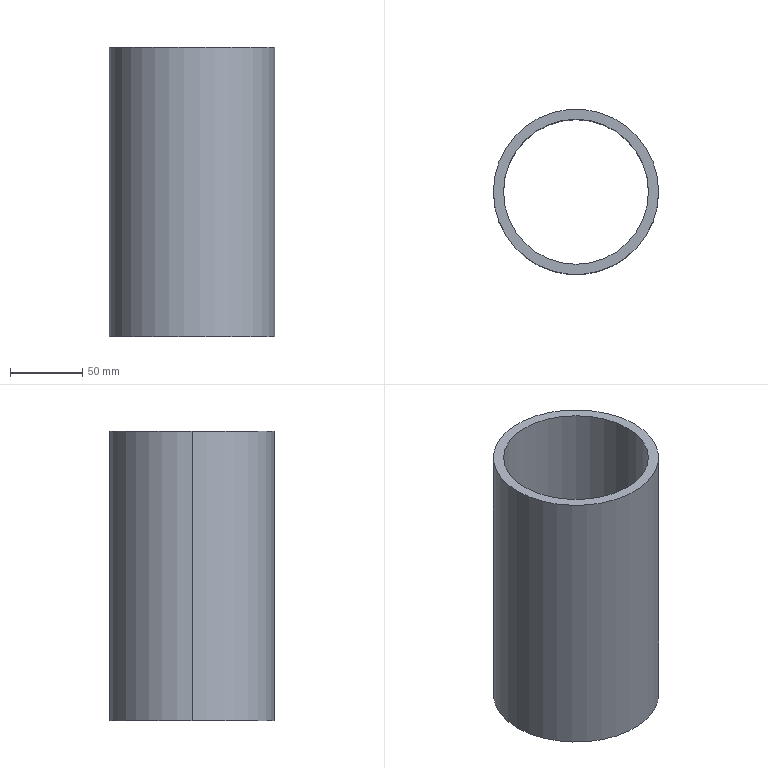Part | SolidWorks | features Extrusion 1, RefAxis 1 | 1 solid | 6 faces | box 114 x 114 x 200 mm | volume 470611 mm3 | cylinder 4 | plane 2 | commonest cylinder face diameters 100 x2 114 x2
STEP:
#1=CARTESIAN_POINT('',(-50.,0.,200.));
#2=VERTEX_POINT('',#1);
#3=CARTESIAN_POINT('',(50.,0.,200.));
#4=VERTEX_POINT('',#3);
#5=CARTESIAN_POINT('',(0.,0.,200.));
#6=DIRECTION('',(0.,0.,1.));
#7=DIRECTION('',(1.,0.,0.));
#8=AXIS2_PLACEMENT_3D('',#5,#6,#7);
#9=CIRCLE('',#8,50.);
#10=EDGE_CURVE('',#2,#4,#9,.T.);
#11=ORIENTED_EDGE('',*,*,#10,.T.);
#12=CARTESIAN_POINT('',(50.,0.,0.));
#13=VERTEX_POINT('',#12);
#14=CARTESIAN_POINT('',(50.,0.,200.));
#15=DIRECTION('',(0.,0.,-1.));
#16=VECTOR('',#15,1000.);
#17=LINE('',#14,#16);
#18=EDGE_CURVE('',#4,#13,#17,.T.);
#19=ORIENTED_EDGE('',*,*,#18,.T.);
#20=CARTESIAN_POINT('',(-50.,0.,0.));
#21=VERTEX_POINT('',#20);
#22=CARTESIAN_POINT('',(0.,0.,0.));
#23=DIRECTION('',(0.,0.,1.));
#24=DIRECTION('',(1.,0.,0.));
#25=AXIS2_PLACEMENT_3D('',#22,#23,#24);
#26=CIRCLE('',#25,50.);
#27=EDGE_CURVE('',#21,#13,#26,.T.);
#28=ORIENTED_EDGE('',*,*,#27,.F.);
#29=CARTESIAN_POINT('',(-50.,0.,200.));
#30=DIRECTION('',(0.,0.,-1.));
#31=VECTOR('',#30,1000.);
#32=LINE('',#29,#31);
#33=EDGE_CURVE('',#2,#21,#32,.T.);
#34=ORIENTED_EDGE('',*,*,#33,.F.);
#35=EDGE_LOOP('',(#11,#19,#28,#34));
#36=FACE_OUTER_BOUND('',#35,.T.);
#37=CARTESIAN_POINT('',(0.,0.,200.));
#38=DIRECTION('',(0.,0.,-1.));
#39=DIRECTION('',(-1.,0.,0.));
#40=AXIS2_PLACEMENT_3D('',#37,#38,#39);
#41=CYLINDRICAL_SURFACE('',#40,50.);
#42=ADVANCED_FACE('',(#36),#41,.F.);
#43=CARTESIAN_POINT('',(57.,0.,200.));
#44=VERTEX_POINT('',#43);
#45=CARTESIAN_POINT('',(-57.,0.,200.));
#46=VERTEX_POINT('',#45);
#47=CARTESIAN_POINT('',(0.,0.,200.));
#48=DIRECTION('',(0.,0.,1.));
#49=DIRECTION('',(1.,0.,0.));
#50=AXIS2_PLACEMENT_3D('',#47,#48,#49);
#51=CIRCLE('',#50,57.);
#52=EDGE_CURVE('',#44,#46,#51,.T.);
#53=ORIENTED_EDGE('',*,*,#52,.F.);
#54=CARTESIAN_POINT('',(57.,0.,0.));
#55=VERTEX_POINT('',#54);
#56=CARTESIAN_POINT('',(57.,0.,200.));
#57=DIRECTION('',(0.,0.,-1.));
#58=VECTOR('',#57,1000.);
#59=LINE('',#56,#58);
#60=EDGE_CURVE('',#44,#55,#59,.T.);
#61=ORIENTED_EDGE('',*,*,#60,.T.);
#62=CARTESIAN_POINT('',(-57.,0.,0.));
#63=VERTEX_POINT('',#62);
#64=CARTESIAN_POINT('',(0.,0.,0.));
#65=DIRECTION('',(0.,0.,1.));
#66=DIRECTION('',(1.,0.,0.));
#67=AXIS2_PLACEMENT_3D('',#64,#65,#66);
#68=CIRCLE('',#67,57.);
#69=EDGE_CURVE('',#55,#63,#68,.T.);
#70=ORIENTED_EDGE('',*,*,#69,.T.);
#71=CARTESIAN_POINT('',(-57.,0.,200.));
#72=DIRECTION('',(0.,0.,-1.));
#73=VECTOR('',#72,1000.);
#74=LINE('',#71,#73);
#75=EDGE_CURVE('',#46,#63,#74,.T.);
#76=ORIENTED_EDGE('',*,*,#75,.F.);
#77=EDGE_LOOP('',(#53,#61,#70,#76));
#78=FACE_OUTER_BOUND('',#77,.T.);
#79=CARTESIAN_POINT('',(0.,0.,200.));
#80=DIRECTION('',(0.,0.,-1.));
#81=DIRECTION('',(-1.,0.,0.));
#82=AXIS2_PLACEMENT_3D('',#79,#80,#81);
#83=CYLINDRICAL_SURFACE('',#82,57.);
#84=ADVANCED_FACE('',(#78),#83,.T.);
#85=CARTESIAN_POINT('',(0.,0.,200.));
#86=DIRECTION('',(0.,0.,1.));
#87=DIRECTION('',(1.,0.,0.));
#88=AXIS2_PLACEMENT_3D('',#85,#86,#87);
#89=CIRCLE('',#88,57.);
#90=EDGE_CURVE('',#46,#44,#89,.T.);
#91=ORIENTED_EDGE('',*,*,#90,.T.);
#92=ORIENTED_EDGE('',*,*,#52,.T.);
#93=EDGE_LOOP('',(#91,#92));
#94=FACE_OUTER_BOUND('',#93,.T.);
#95=ORIENTED_EDGE('',*,*,#10,.F.);
#96=CARTESIAN_POINT('',(0.,0.,200.));
#97=DIRECTION('',(0.,0.,1.));
#98=DIRECTION('',(1.,0.,0.));
#99=AXIS2_PLACEMENT_3D('',#96,#97,#98);
#100=CIRCLE('',#99,50.);
#101=EDGE_CURVE('',#4,#2,#100,.T.);
#102=ORIENTED_EDGE('',*,*,#101,.F.);
#103=EDGE_LOOP('',(#95,#102));
#104=FACE_BOUND('',#103,.T.);
#105=CARTESIAN_POINT('',(0.,0.,200.));
#106=DIRECTION('',(0.,0.,1.));
#107=DIRECTION('',(1.,0.,0.));
#108=AXIS2_PLACEMENT_3D('',#105,#106,#107);
#109=PLANE('',#108);
#110=ADVANCED_FACE('',(#94,#104),#109,.T.);
#111=CARTESIAN_POINT('',(0.,0.,0.));
#112=DIRECTION('',(0.,0.,1.));
#113=DIRECTION('',(1.,0.,0.));
#114=AXIS2_PLACEMENT_3D('',#111,#112,#113);
#115=CIRCLE('',#114,57.);
#116=EDGE_CURVE('',#63,#55,#115,.T.);
#117=ORIENTED_EDGE('',*,*,#116,.F.);
#118=ORIENTED_EDGE('',*,*,#69,.F.);
#119=EDGE_LOOP('',(#117,#118));
#120=FACE_OUTER_BOUND('',#119,.T.);
#121=ORIENTED_EDGE('',*,*,#27,.T.);
#122=CARTESIAN_POINT('',(0.,0.,0.));
#123=DIRECTION('',(0.,0.,1.));
#124=DIRECTION('',(1.,0.,0.));
#125=AXIS2_PLACEMENT_3D('',#122,#123,#124);
#126=CIRCLE('',#125,50.);
#127=EDGE_CURVE('',#13,#21,#126,.T.);
#128=ORIENTED_EDGE('',*,*,#127,.T.);
#129=EDGE_LOOP('',(#121,#128));
#130=FACE_BOUND('',#129,.T.);
#131=CARTESIAN_POINT('',(0.,0.,0.));
#132=DIRECTION('',(0.,0.,1.));
#133=DIRECTION('',(1.,0.,0.));
#134=AXIS2_PLACEMENT_3D('',#131,#132,#133);
#135=PLANE('',#134);
#136=ADVANCED_FACE('',(#120,#130),#135,.F.);
#137=ORIENTED_EDGE('',*,*,#60,.F.);
#138=ORIENTED_EDGE('',*,*,#90,.F.);
#139=ORIENTED_EDGE('',*,*,#75,.T.);
#140=ORIENTED_EDGE('',*,*,#116,.T.);
#141=EDGE_LOOP('',(#137,#138,#139,#140));
#142=FACE_OUTER_BOUND('',#141,.T.);
#143=CARTESIAN_POINT('',(0.,0.,200.));
#144=DIRECTION('',(0.,0.,-1.));
#145=DIRECTION('',(-1.,0.,0.));
#146=AXIS2_PLACEMENT_3D('',#143,#144,#145);
#147=CYLINDRICAL_SURFACE('',#146,57.);
#148=ADVANCED_FACE('',(#142),#147,.T.);
#149=ORIENTED_EDGE('',*,*,#18,.F.);
#150=ORIENTED_EDGE('',*,*,#101,.T.);
#151=ORIENTED_EDGE('',*,*,#33,.T.);
#152=ORIENTED_EDGE('',*,*,#127,.F.);
#153=EDGE_LOOP('',(#149,#150,#151,#152));
#154=FACE_OUTER_BOUND('',#153,.T.);
#155=CARTESIAN_POINT('',(0.,0.,200.));
#156=DIRECTION('',(0.,0.,-1.));
#157=DIRECTION('',(-1.,0.,0.));
#158=AXIS2_PLACEMENT_3D('',#155,#156,#157);
#159=CYLINDRICAL_SURFACE('',#158,50.);
#160=ADVANCED_FACE('',(#154),#159,.F.);
#161=CLOSED_SHELL('',(#42,#84,#110,#136,#148,#160));
#162=MANIFOLD_SOLID_BREP('',#161);
#163=CARTESIAN_POINT('',(0.,0.,0.));
#164=DIRECTION('',(0.,0.,1.));
#165=DIRECTION('',(1.,0.,0.));
#166=AXIS2_PLACEMENT_3D('',#163,#164,#165);
#167=(LENGTH_UNIT()NAMED_UNIT(*)SI_UNIT(.MILLI.,.METRE.));
#168=UNCERTAINTY_MEASURE_WITH_UNIT(LENGTH_MEASURE(0.00001),#167,'','');
#169=(NAMED_UNIT(*)PLANE_ANGLE_UNIT()SI_UNIT($,.RADIAN.));
#170=(NAMED_UNIT(*)SI_UNIT($,.STERADIAN.)SOLID_ANGLE_UNIT());
#171=(GEOMETRIC_REPRESENTATION_CONTEXT(3)GLOBAL_UNCERTAINTY_ASSIGNED_CONTEXT((#168))GLOBAL_UNIT_ASSIGNED_CONTEXT((#167,#169,#170))REPRESENTATION_CONTEXT('',''));
#172=ADVANCED_BREP_SHAPE_REPRESENTATION('',(#162,#166),#171);